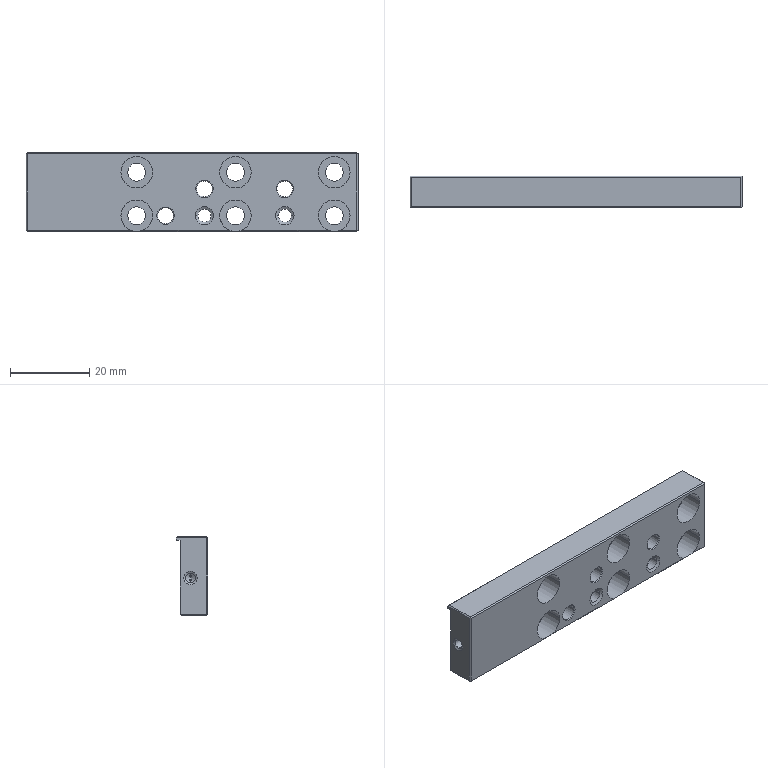Part | NX | 1 solid | 79 faces | box 84 x 8 x 20 mm | volume 9591 mm3 | cylinder 38 | plane 27 | cone 14 | commonest cylinder face diameters 4.5 x12 8 x12 4 x6 2.5 x4 3.3 x4